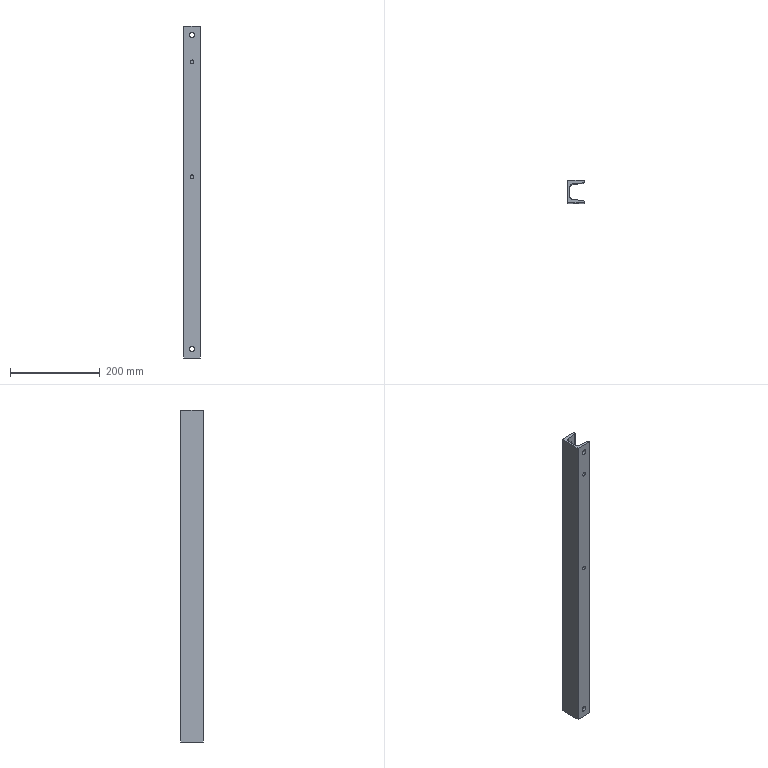Part | STEP file | HESS-408-70-15W-W-40-5# channel 2_default_machined_ | 1 solid | 26 faces | box 37 x 50 x 740 mm | volume 497631 mm3 | cylinder 16 | plane 10 | commonest cylinder face diameters 12 x8 8.5 x4 7 x2 14 x2